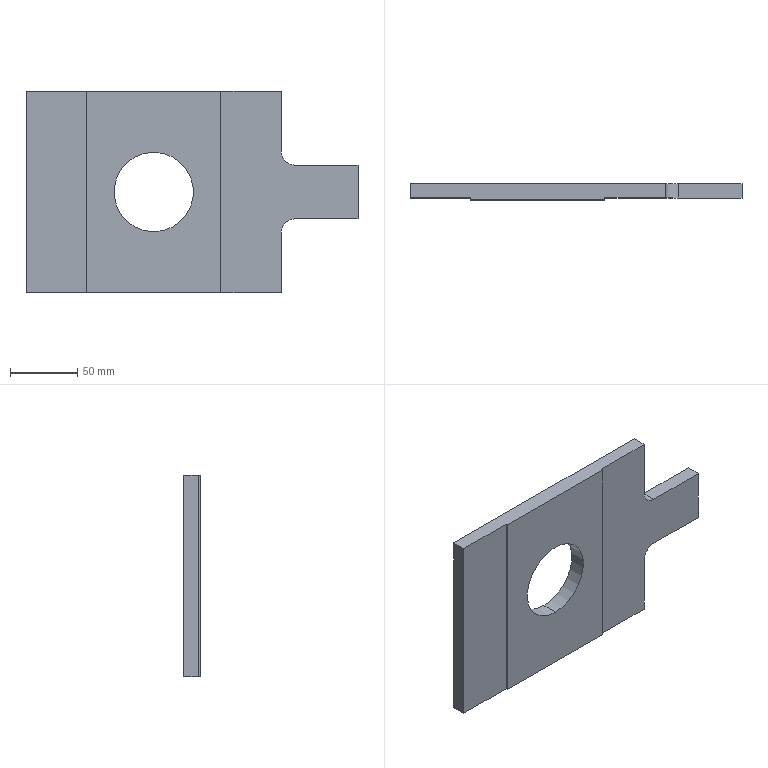Part | SolidWorks | features ICE 2, Extrusion 1, Fillet 1 | 1 solid | 18 faces | box 247 x 12 x 150 mm | volume 313333 mm3 | plane 14 | cylinder 4 | commonest cylinder face diameters 20 x2 59 x2
STEP:
#1=CARTESIAN_POINT('',(0.,0.,29.5));
#2=VERTEX_POINT('',#1);
#3=CARTESIAN_POINT('',(0.,0.,-29.5));
#4=VERTEX_POINT('',#3);
#5=CARTESIAN_POINT('',(0.,0.,0.));
#6=DIRECTION('',(0.,-1.,0.));
#7=DIRECTION('',(0.,0.,1.));
#8=AXIS2_PLACEMENT_3D('',#5,#6,#7);
#9=CIRCLE('',#8,29.5);
#10=EDGE_CURVE('',#2,#4,#9,.T.);
#11=ORIENTED_EDGE('',*,*,#10,.T.);
#12=CARTESIAN_POINT('',(0.,12.,-29.5));
#13=VERTEX_POINT('',#12);
#14=CARTESIAN_POINT('',(0.,-0.001,-29.5));
#15=DIRECTION('',(0.,1.,0.));
#16=VECTOR('',#15,1000.);
#17=LINE('',#14,#16);
#18=EDGE_CURVE('',#4,#13,#17,.T.);
#19=ORIENTED_EDGE('',*,*,#18,.T.);
#20=CARTESIAN_POINT('',(0.,12.,29.5));
#21=VERTEX_POINT('',#20);
#22=CARTESIAN_POINT('',(0.,12.,0.));
#23=DIRECTION('',(0.,1.,0.));
#24=DIRECTION('',(0.,0.,1.));
#25=AXIS2_PLACEMENT_3D('',#22,#23,#24);
#26=CIRCLE('',#25,29.5);
#27=EDGE_CURVE('',#13,#21,#26,.T.);
#28=ORIENTED_EDGE('',*,*,#27,.T.);
#29=CARTESIAN_POINT('',(0.,-0.001,29.5));
#30=DIRECTION('',(0.,1.,0.));
#31=VECTOR('',#30,1000.);
#32=LINE('',#29,#31);
#33=EDGE_CURVE('',#2,#21,#32,.T.);
#34=ORIENTED_EDGE('',*,*,#33,.F.);
#35=EDGE_LOOP('',(#11,#19,#28,#34));
#36=FACE_OUTER_BOUND('',#35,.T.);
#37=CARTESIAN_POINT('',(0.,-0.001,0.));
#38=DIRECTION('',(0.,1.,0.));
#39=DIRECTION('',(0.,0.,1.));
#40=AXIS2_PLACEMENT_3D('',#37,#38,#39);
#41=CYLINDRICAL_SURFACE('',#40,29.5);
#42=ADVANCED_FACE('',(#36),#41,.F.);
#43=CARTESIAN_POINT('',(95.,1.5,75.));
#44=VERTEX_POINT('',#43);
#45=CARTESIAN_POINT('',(95.,1.5,30.));
#46=VERTEX_POINT('',#45);
#47=CARTESIAN_POINT('',(95.,1.5,75.));
#48=DIRECTION('',(0.,0.,-1.));
#49=VECTOR('',#48,1000.);
#50=LINE('',#47,#49);
#51=EDGE_CURVE('',#44,#46,#50,.T.);
#52=ORIENTED_EDGE('',*,*,#51,.T.);
#53=CARTESIAN_POINT('',(95.,12.,30.));
#54=VERTEX_POINT('',#53);
#55=CARTESIAN_POINT('',(95.,12.,30.));
#56=DIRECTION('',(0.,1.,0.));
#57=VECTOR('',#56,1000.);
#58=LINE('',#55,#57);
#59=EDGE_CURVE('',#46,#54,#58,.T.);
#60=ORIENTED_EDGE('',*,*,#59,.T.);
#61=CARTESIAN_POINT('',(95.,12.,75.));
#62=VERTEX_POINT('',#61);
#63=CARTESIAN_POINT('',(95.,12.,75.));
#64=DIRECTION('',(0.,0.,-1.));
#65=VECTOR('',#64,1000.);
#66=LINE('',#63,#65);
#67=EDGE_CURVE('',#62,#54,#66,.T.);
#68=ORIENTED_EDGE('',*,*,#67,.F.);
#69=CARTESIAN_POINT('',(95.,12.,75.));
#70=DIRECTION('',(0.,1.,0.));
#71=VECTOR('',#70,1000.);
#72=LINE('',#69,#71);
#73=EDGE_CURVE('',#44,#62,#72,.T.);
#74=ORIENTED_EDGE('',*,*,#73,.F.);
#75=EDGE_LOOP('',(#52,#60,#68,#74));
#76=FACE_OUTER_BOUND('',#75,.T.);
#77=CARTESIAN_POINT('',(95.,12.,75.));
#78=DIRECTION('',(-1.,0.,0.));
#79=DIRECTION('',(0.,0.,1.));
#80=AXIS2_PLACEMENT_3D('',#77,#78,#79);
#81=PLANE('',#80);
#82=ADVANCED_FACE('',(#76),#81,.F.);
#83=CARTESIAN_POINT('',(95.,12.,-30.));
#84=VERTEX_POINT('',#83);
#85=CARTESIAN_POINT('',(95.,12.,-75.));
#86=VERTEX_POINT('',#85);
#87=CARTESIAN_POINT('',(95.,12.,75.));
#88=DIRECTION('',(0.,0.,-1.));
#89=VECTOR('',#88,1000.);
#90=LINE('',#87,#89);
#91=EDGE_CURVE('',#84,#86,#90,.T.);
#92=ORIENTED_EDGE('',*,*,#91,.F.);
#93=CARTESIAN_POINT('',(95.,1.5,-30.));
#94=VERTEX_POINT('',#93);
#95=CARTESIAN_POINT('',(95.,1.5,-30.));
#96=DIRECTION('',(0.,-1.,0.));
#97=VECTOR('',#96,1000.);
#98=LINE('',#95,#97);
#99=EDGE_CURVE('',#84,#94,#98,.T.);
#100=ORIENTED_EDGE('',*,*,#99,.T.);
#101=CARTESIAN_POINT('',(95.,1.5,-75.));
#102=VERTEX_POINT('',#101);
#103=CARTESIAN_POINT('',(95.,1.5,75.));
#104=DIRECTION('',(0.,0.,-1.));
#105=VECTOR('',#104,1000.);
#106=LINE('',#103,#105);
#107=EDGE_CURVE('',#94,#102,#106,.T.);
#108=ORIENTED_EDGE('',*,*,#107,.T.);
#109=CARTESIAN_POINT('',(95.,12.,-75.));
#110=DIRECTION('',(0.,1.,0.));
#111=VECTOR('',#110,1000.);
#112=LINE('',#109,#111);
#113=EDGE_CURVE('',#102,#86,#112,.T.);
#114=ORIENTED_EDGE('',*,*,#113,.T.);
#115=EDGE_LOOP('',(#92,#100,#108,#114));
#116=FACE_OUTER_BOUND('',#115,.T.);
#117=CARTESIAN_POINT('',(95.,12.,75.));
#118=DIRECTION('',(-1.,0.,0.));
#119=DIRECTION('',(0.,0.,1.));
#120=AXIS2_PLACEMENT_3D('',#117,#118,#119);
#121=PLANE('',#120);
#122=ADVANCED_FACE('',(#116),#121,.F.);
#123=CARTESIAN_POINT('',(50.,0.,-75.));
#124=VERTEX_POINT('',#123);
#125=CARTESIAN_POINT('',(50.,1.5,-75.));
#126=VERTEX_POINT('',#125);
#127=CARTESIAN_POINT('',(50.,1.5,-75.));
#128=DIRECTION('',(0.,1.,0.));
#129=VECTOR('',#128,1000.);
#130=LINE('',#127,#129);
#131=EDGE_CURVE('',#124,#126,#130,.T.);
#132=ORIENTED_EDGE('',*,*,#131,.T.);
#133=CARTESIAN_POINT('',(50.,1.5,75.));
#134=VERTEX_POINT('',#133);
#135=CARTESIAN_POINT('',(50.,1.5,75.));
#136=DIRECTION('',(0.,0.,-1.));
#137=VECTOR('',#136,1000.);
#138=LINE('',#135,#137);
#139=EDGE_CURVE('',#134,#126,#138,.T.);
#140=ORIENTED_EDGE('',*,*,#139,.F.);
#141=CARTESIAN_POINT('',(50.,0.,75.));
#142=VERTEX_POINT('',#141);
#143=CARTESIAN_POINT('',(50.,1.5,75.));
#144=DIRECTION('',(0.,1.,0.));
#145=VECTOR('',#144,1000.);
#146=LINE('',#143,#145);
#147=EDGE_CURVE('',#142,#134,#146,.T.);
#148=ORIENTED_EDGE('',*,*,#147,.F.);
#149=CARTESIAN_POINT('',(50.,0.,75.));
#150=DIRECTION('',(0.,0.,-1.));
#151=VECTOR('',#150,1000.);
#152=LINE('',#149,#151);
#153=EDGE_CURVE('',#142,#124,#152,.T.);
#154=ORIENTED_EDGE('',*,*,#153,.T.);
#155=EDGE_LOOP('',(#132,#140,#148,#154));
#156=FACE_OUTER_BOUND('',#155,.T.);
#157=CARTESIAN_POINT('',(50.,1.5,75.));
#158=DIRECTION('',(-1.,0.,0.));
#159=DIRECTION('',(0.,0.,1.));
#160=AXIS2_PLACEMENT_3D('',#157,#158,#159);
#161=PLANE('',#160);
#162=ADVANCED_FACE('',(#156),#161,.F.);
#163=CARTESIAN_POINT('',(95.,1.5,-75.));
#164=DIRECTION('',(1.,0.,0.));
#165=VECTOR('',#164,1000.);
#166=LINE('',#163,#165);
#167=EDGE_CURVE('',#126,#102,#166,.T.);
#168=ORIENTED_EDGE('',*,*,#167,.T.);
#169=ORIENTED_EDGE('',*,*,#107,.F.);
#170=CARTESIAN_POINT('',(105.,1.5,-20.));
#171=VERTEX_POINT('',#170);
#172=CARTESIAN_POINT('',(105.,1.5,-30.));
#173=DIRECTION('',(0.,1.,0.));
#174=DIRECTION('',(0.,0.,1.));
#175=AXIS2_PLACEMENT_3D('',#172,#173,#174);
#176=CIRCLE('',#175,10.);
#177=EDGE_CURVE('',#94,#171,#176,.T.);
#178=ORIENTED_EDGE('',*,*,#177,.T.);
#179=CARTESIAN_POINT('',(152.,1.5,-20.));
#180=VERTEX_POINT('',#179);
#181=CARTESIAN_POINT('',(152.,1.5,-20.));
#182=DIRECTION('',(-1.,0.,0.));
#183=VECTOR('',#182,1000.);
#184=LINE('',#181,#183);
#185=EDGE_CURVE('',#180,#171,#184,.T.);
#186=ORIENTED_EDGE('',*,*,#185,.F.);
#187=CARTESIAN_POINT('',(152.,1.5,20.));
#188=VERTEX_POINT('',#187);
#189=CARTESIAN_POINT('',(152.,1.5,20.));
#190=DIRECTION('',(0.,0.,-1.));
#191=VECTOR('',#190,1000.);
#192=LINE('',#189,#191);
#193=EDGE_CURVE('',#188,#180,#192,.T.);
#194=ORIENTED_EDGE('',*,*,#193,.F.);
#195=CARTESIAN_POINT('',(105.,1.5,20.));
#196=VERTEX_POINT('',#195);
#197=CARTESIAN_POINT('',(152.,1.5,20.));
#198=DIRECTION('',(-1.,0.,0.));
#199=VECTOR('',#198,1000.);
#200=LINE('',#197,#199);
#201=EDGE_CURVE('',#188,#196,#200,.T.);
#202=ORIENTED_EDGE('',*,*,#201,.T.);
#203=CARTESIAN_POINT('',(105.,1.5,30.));
#204=DIRECTION('',(0.,1.,0.));
#205=DIRECTION('',(0.,0.,1.));
#206=AXIS2_PLACEMENT_3D('',#203,#204,#205);
#207=CIRCLE('',#206,10.);
#208=EDGE_CURVE('',#196,#46,#207,.T.);
#209=ORIENTED_EDGE('',*,*,#208,.T.);
#210=ORIENTED_EDGE('',*,*,#51,.F.);
#211=CARTESIAN_POINT('',(95.,1.5,75.));
#212=DIRECTION('',(1.,0.,0.));
#213=VECTOR('',#212,1000.);
#214=LINE('',#211,#213);
#215=EDGE_CURVE('',#134,#44,#214,.T.);
#216=ORIENTED_EDGE('',*,*,#215,.F.);
#217=ORIENTED_EDGE('',*,*,#139,.T.);
#218=EDGE_LOOP('',(#168,#169,#178,#186,#194,#202,#209,#210,#216,#217));
#219=FACE_OUTER_BOUND('',#218,.T.);
#220=CARTESIAN_POINT('',(95.,1.5,75.));
#221=DIRECTION('',(0.,1.,0.));
#222=DIRECTION('',(0.,0.,1.));
#223=AXIS2_PLACEMENT_3D('',#220,#221,#222);
#224=PLANE('',#223);
#225=ADVANCED_FACE('',(#219),#224,.F.);
#226=CARTESIAN_POINT('',(0.,12.,0.));
#227=DIRECTION('',(0.,1.,0.));
#228=DIRECTION('',(0.,0.,1.));
#229=AXIS2_PLACEMENT_3D('',#226,#227,#228);
#230=CIRCLE('',#229,29.5);
#231=EDGE_CURVE('',#21,#13,#230,.T.);
#232=ORIENTED_EDGE('',*,*,#231,.F.);
#233=ORIENTED_EDGE('',*,*,#27,.F.);
#234=EDGE_LOOP('',(#232,#233));
#235=FACE_BOUND('',#234,.T.);
#236=CARTESIAN_POINT('',(-95.,12.,-75.));
#237=VERTEX_POINT('',#236);
#238=CARTESIAN_POINT('',(-95.,12.,-75.));
#239=DIRECTION('',(-1.,0.,0.));
#240=VECTOR('',#239,1000.);
#241=LINE('',#238,#240);
#242=EDGE_CURVE('',#86,#237,#241,.T.);
#243=ORIENTED_EDGE('',*,*,#242,.T.);
#244=CARTESIAN_POINT('',(-95.,12.,75.));
#245=VERTEX_POINT('',#244);
#246=CARTESIAN_POINT('',(-95.,12.,75.));
#247=DIRECTION('',(0.,0.,-1.));
#248=VECTOR('',#247,1000.);
#249=LINE('',#246,#248);
#250=EDGE_CURVE('',#245,#237,#249,.T.);
#251=ORIENTED_EDGE('',*,*,#250,.F.);
#252=CARTESIAN_POINT('',(-95.,12.,75.));
#253=DIRECTION('',(-1.,0.,0.));
#254=VECTOR('',#253,1000.);
#255=LINE('',#252,#254);
#256=EDGE_CURVE('',#62,#245,#255,.T.);
#257=ORIENTED_EDGE('',*,*,#256,.F.);
#258=ORIENTED_EDGE('',*,*,#67,.T.);
#259=CARTESIAN_POINT('',(105.,12.,20.));
#260=VERTEX_POINT('',#259);
#261=CARTESIAN_POINT('',(105.,12.,30.));
#262=DIRECTION('',(0.,-1.,0.));
#263=DIRECTION('',(0.,0.,-1.));
#264=AXIS2_PLACEMENT_3D('',#261,#262,#263);
#265=CIRCLE('',#264,10.);
#266=EDGE_CURVE('',#54,#260,#265,.T.);
#267=ORIENTED_EDGE('',*,*,#266,.T.);
#268=CARTESIAN_POINT('',(152.,12.,20.));
#269=VERTEX_POINT('',#268);
#270=CARTESIAN_POINT('',(152.,12.,20.));
#271=DIRECTION('',(-1.,0.,0.));
#272=VECTOR('',#271,1000.);
#273=LINE('',#270,#272);
#274=EDGE_CURVE('',#269,#260,#273,.T.);
#275=ORIENTED_EDGE('',*,*,#274,.F.);
#276=CARTESIAN_POINT('',(152.,12.,-20.));
#277=VERTEX_POINT('',#276);
#278=CARTESIAN_POINT('',(152.,12.,20.));
#279=DIRECTION('',(0.,0.,1.));
#280=VECTOR('',#279,1000.);
#281=LINE('',#278,#280);
#282=EDGE_CURVE('',#277,#269,#281,.T.);
#283=ORIENTED_EDGE('',*,*,#282,.F.);
#284=CARTESIAN_POINT('',(105.,12.,-20.));
#285=VERTEX_POINT('',#284);
#286=CARTESIAN_POINT('',(152.,12.,-20.));
#287=DIRECTION('',(-1.,0.,0.));
#288=VECTOR('',#287,1000.);
#289=LINE('',#286,#288);
#290=EDGE_CURVE('',#277,#285,#289,.T.);
#291=ORIENTED_EDGE('',*,*,#290,.T.);
#292=CARTESIAN_POINT('',(105.,12.,-30.));
#293=DIRECTION('',(0.,-1.,0.));
#294=DIRECTION('',(0.,0.,-1.));
#295=AXIS2_PLACEMENT_3D('',#292,#293,#294);
#296=CIRCLE('',#295,10.);
#297=EDGE_CURVE('',#285,#84,#296,.T.);
#298=ORIENTED_EDGE('',*,*,#297,.T.);
#299=ORIENTED_EDGE('',*,*,#91,.T.);
#300=EDGE_LOOP('',(#243,#251,#257,#258,#267,#275,#283,#291,#298,#299));
#301=FACE_OUTER_BOUND('',#300,.T.);
#302=CARTESIAN_POINT('',(-95.,12.,75.));
#303=DIRECTION('',(0.,-1.,0.));
#304=DIRECTION('',(0.,0.,-1.));
#305=AXIS2_PLACEMENT_3D('',#302,#303,#304);
#306=PLANE('',#305);
#307=ADVANCED_FACE('',(#235,#301),#306,.F.);
#308=CARTESIAN_POINT('',(-95.,1.5,-75.));
#309=VERTEX_POINT('',#308);
#310=CARTESIAN_POINT('',(-95.,1.5,-75.));
#311=DIRECTION('',(0.,-1.,0.));
#312=VECTOR('',#311,1000.);
#313=LINE('',#310,#312);
#314=EDGE_CURVE('',#237,#309,#313,.T.);
#315=ORIENTED_EDGE('',*,*,#314,.T.);
#316=CARTESIAN_POINT('',(-95.,1.5,75.));
#317=VERTEX_POINT('',#316);
#318=CARTESIAN_POINT('',(-95.,1.5,75.));
#319=DIRECTION('',(0.,0.,-1.));
#320=VECTOR('',#319,1000.);
#321=LINE('',#318,#320);
#322=EDGE_CURVE('',#317,#309,#321,.T.);
#323=ORIENTED_EDGE('',*,*,#322,.F.);
#324=CARTESIAN_POINT('',(-95.,1.5,75.));
#325=DIRECTION('',(0.,-1.,0.));
#326=VECTOR('',#325,1000.);
#327=LINE('',#324,#326);
#328=EDGE_CURVE('',#245,#317,#327,.T.);
#329=ORIENTED_EDGE('',*,*,#328,.F.);
#330=ORIENTED_EDGE('',*,*,#250,.T.);
#331=EDGE_LOOP('',(#315,#323,#329,#330));
#332=FACE_OUTER_BOUND('',#331,.T.);
#333=CARTESIAN_POINT('',(-95.,1.5,75.));
#334=DIRECTION('',(1.,0.,0.));
#335=DIRECTION('',(0.,0.,-1.));
#336=AXIS2_PLACEMENT_3D('',#333,#334,#335);
#337=PLANE('',#336);
#338=ADVANCED_FACE('',(#332),#337,.F.);
#339=CARTESIAN_POINT('',(-50.,1.5,-75.));
#340=VERTEX_POINT('',#339);
#341=CARTESIAN_POINT('',(-50.,1.5,-75.));
#342=DIRECTION('',(1.,0.,0.));
#343=VECTOR('',#342,1000.);
#344=LINE('',#341,#343);
#345=EDGE_CURVE('',#309,#340,#344,.T.);
#346=ORIENTED_EDGE('',*,*,#345,.T.);
#347=CARTESIAN_POINT('',(-50.,1.5,75.));
#348=VERTEX_POINT('',#347);
#349=CARTESIAN_POINT('',(-50.,1.5,75.));
#350=DIRECTION('',(0.,0.,-1.));
#351=VECTOR('',#350,1000.);
#352=LINE('',#349,#351);
#353=EDGE_CURVE('',#348,#340,#352,.T.);
#354=ORIENTED_EDGE('',*,*,#353,.F.);
#355=CARTESIAN_POINT('',(-50.,1.5,75.));
#356=DIRECTION('',(1.,0.,0.));
#357=VECTOR('',#356,1000.);
#358=LINE('',#355,#357);
#359=EDGE_CURVE('',#317,#348,#358,.T.);
#360=ORIENTED_EDGE('',*,*,#359,.F.);
#361=ORIENTED_EDGE('',*,*,#322,.T.);
#362=EDGE_LOOP('',(#346,#354,#360,#361));
#363=FACE_OUTER_BOUND('',#362,.T.);
#364=CARTESIAN_POINT('',(-50.,1.5,75.));
#365=DIRECTION('',(0.,1.,0.));
#366=DIRECTION('',(0.,0.,1.));
#367=AXIS2_PLACEMENT_3D('',#364,#365,#366);
#368=PLANE('',#367);
#369=ADVANCED_FACE('',(#363),#368,.F.);
#370=CARTESIAN_POINT('',(-50.,0.,-75.));
#371=VERTEX_POINT('',#370);
#372=CARTESIAN_POINT('',(-50.,0.,-75.));
#373=DIRECTION('',(0.,-1.,0.));
#374=VECTOR('',#373,1000.);
#375=LINE('',#372,#374);
#376=EDGE_CURVE('',#340,#371,#375,.T.);
#377=ORIENTED_EDGE('',*,*,#376,.T.);
#378=CARTESIAN_POINT('',(-50.,0.,75.));
#379=VERTEX_POINT('',#378);
#380=CARTESIAN_POINT('',(-50.,0.,75.));
#381=DIRECTION('',(0.,0.,-1.));
#382=VECTOR('',#381,1000.);
#383=LINE('',#380,#382);
#384=EDGE_CURVE('',#379,#371,#383,.T.);
#385=ORIENTED_EDGE('',*,*,#384,.F.);
#386=CARTESIAN_POINT('',(-50.,0.,75.));
#387=DIRECTION('',(0.,-1.,0.));
#388=VECTOR('',#387,1000.);
#389=LINE('',#386,#388);
#390=EDGE_CURVE('',#348,#379,#389,.T.);
#391=ORIENTED_EDGE('',*,*,#390,.F.);
#392=ORIENTED_EDGE('',*,*,#353,.T.);
#393=EDGE_LOOP('',(#377,#385,#391,#392));
#394=FACE_OUTER_BOUND('',#393,.T.);
#395=CARTESIAN_POINT('',(-50.,0.,75.));
#396=DIRECTION('',(1.,0.,0.));
#397=DIRECTION('',(0.,1.,0.));
#398=AXIS2_PLACEMENT_3D('',#395,#396,#397);
#399=PLANE('',#398);
#400=ADVANCED_FACE('',(#394),#399,.F.);
#401=ORIENTED_EDGE('',*,*,#10,.F.);
#402=CARTESIAN_POINT('',(0.,0.,0.));
#403=DIRECTION('',(0.,-1.,0.));
#404=DIRECTION('',(0.,0.,1.));
#405=AXIS2_PLACEMENT_3D('',#402,#403,#404);
#406=CIRCLE('',#405,29.5);
#407=EDGE_CURVE('',#4,#2,#406,.T.);
#408=ORIENTED_EDGE('',*,*,#407,.F.);
#409=EDGE_LOOP('',(#401,#408));
#410=FACE_BOUND('',#409,.T.);
#411=CARTESIAN_POINT('',(0.,0.,-75.));
#412=DIRECTION('',(1.,0.,0.));
#413=VECTOR('',#412,1000.);
#414=LINE('',#411,#413);
#415=EDGE_CURVE('',#371,#124,#414,.T.);
#416=ORIENTED_EDGE('',*,*,#415,.T.);
#417=ORIENTED_EDGE('',*,*,#153,.F.);
#418=CARTESIAN_POINT('',(50.,0.,75.));
#419=DIRECTION('',(1.,0.,0.));
#420=VECTOR('',#419,1000.);
#421=LINE('',#418,#420);
#422=EDGE_CURVE('',#379,#142,#421,.T.);
#423=ORIENTED_EDGE('',*,*,#422,.F.);
#424=ORIENTED_EDGE('',*,*,#384,.T.);
#425=EDGE_LOOP('',(#416,#417,#423,#424));
#426=FACE_OUTER_BOUND('',#425,.T.);
#427=CARTESIAN_POINT('',(0.,0.,75.));
#428=DIRECTION('',(0.,1.,0.));
#429=DIRECTION('',(0.,0.,1.));
#430=AXIS2_PLACEMENT_3D('',#427,#428,#429);
#431=PLANE('',#430);
#432=ADVANCED_FACE('',(#410,#426),#431,.F.);
#433=ORIENTED_EDGE('',*,*,#422,.T.);
#434=ORIENTED_EDGE('',*,*,#147,.T.);
#435=ORIENTED_EDGE('',*,*,#215,.T.);
#436=ORIENTED_EDGE('',*,*,#73,.T.);
#437=ORIENTED_EDGE('',*,*,#256,.T.);
#438=ORIENTED_EDGE('',*,*,#328,.T.);
#439=ORIENTED_EDGE('',*,*,#359,.T.);
#440=ORIENTED_EDGE('',*,*,#390,.T.);
#441=EDGE_LOOP('',(#433,#434,#435,#436,#437,#438,#439,#440));
#442=FACE_OUTER_BOUND('',#441,.T.);
#443=CARTESIAN_POINT('',(0.,0.,75.));
#444=DIRECTION('',(0.,0.,-1.));
#445=DIRECTION('',(-1.,0.,0.));
#446=AXIS2_PLACEMENT_3D('',#443,#444,#445);
#447=PLANE('',#446);
#448=ADVANCED_FACE('',(#442),#447,.F.);
#449=ORIENTED_EDGE('',*,*,#131,.F.);
#450=ORIENTED_EDGE('',*,*,#415,.F.);
#451=ORIENTED_EDGE('',*,*,#376,.F.);
#452=ORIENTED_EDGE('',*,*,#345,.F.);
#453=ORIENTED_EDGE('',*,*,#314,.F.);
#454=ORIENTED_EDGE('',*,*,#242,.F.);
#455=ORIENTED_EDGE('',*,*,#113,.F.);
#456=ORIENTED_EDGE('',*,*,#167,.F.);
#457=EDGE_LOOP('',(#449,#450,#451,#452,#453,#454,#455,#456));
#458=FACE_OUTER_BOUND('',#457,.T.);
#459=CARTESIAN_POINT('',(0.,0.,-75.));
#460=DIRECTION('',(0.,0.,-1.));
#461=DIRECTION('',(-1.,0.,0.));
#462=AXIS2_PLACEMENT_3D('',#459,#460,#461);
#463=PLANE('',#462);
#464=ADVANCED_FACE('',(#458),#463,.T.);
#465=ORIENTED_EDGE('',*,*,#18,.F.);
#466=ORIENTED_EDGE('',*,*,#407,.T.);
#467=ORIENTED_EDGE('',*,*,#33,.T.);
#468=ORIENTED_EDGE('',*,*,#231,.T.);
#469=EDGE_LOOP('',(#465,#466,#467,#468));
#470=FACE_OUTER_BOUND('',#469,.T.);
#471=CARTESIAN_POINT('',(0.,-0.001,0.));
#472=DIRECTION('',(0.,1.,0.));
#473=DIRECTION('',(0.,0.,1.));
#474=AXIS2_PLACEMENT_3D('',#471,#472,#473);
#475=CYLINDRICAL_SURFACE('',#474,29.5);
#476=ADVANCED_FACE('',(#470),#475,.F.);
#477=ORIENTED_EDGE('',*,*,#274,.T.);
#478=CARTESIAN_POINT('',(105.,1.5,20.));
#479=DIRECTION('',(0.,-1.,0.));
#480=VECTOR('',#479,1000.);
#481=LINE('',#478,#480);
#482=EDGE_CURVE('',#260,#196,#481,.T.);
#483=ORIENTED_EDGE('',*,*,#482,.T.);
#484=ORIENTED_EDGE('',*,*,#201,.F.);
#485=CARTESIAN_POINT('',(152.,12.,20.));
#486=DIRECTION('',(0.,-1.,0.));
#487=VECTOR('',#486,1000.);
#488=LINE('',#485,#487);
#489=EDGE_CURVE('',#269,#188,#488,.T.);
#490=ORIENTED_EDGE('',*,*,#489,.F.);
#491=EDGE_LOOP('',(#477,#483,#484,#490));
#492=FACE_OUTER_BOUND('',#491,.T.);
#493=CARTESIAN_POINT('',(152.,12.,20.));
#494=DIRECTION('',(0.,0.,-1.));
#495=DIRECTION('',(-1.,0.,0.));
#496=AXIS2_PLACEMENT_3D('',#493,#494,#495);
#497=PLANE('',#496);
#498=ADVANCED_FACE('',(#492),#497,.F.);
#499=ORIENTED_EDGE('',*,*,#185,.T.);
#500=CARTESIAN_POINT('',(105.,12.,-20.));
#501=DIRECTION('',(0.,1.,0.));
#502=VECTOR('',#501,1000.);
#503=LINE('',#500,#502);
#504=EDGE_CURVE('',#171,#285,#503,.T.);
#505=ORIENTED_EDGE('',*,*,#504,.T.);
#506=ORIENTED_EDGE('',*,*,#290,.F.);
#507=CARTESIAN_POINT('',(152.,12.,-20.));
#508=DIRECTION('',(0.,1.,0.));
#509=VECTOR('',#508,1000.);
#510=LINE('',#507,#509);
#511=EDGE_CURVE('',#180,#277,#510,.T.);
#512=ORIENTED_EDGE('',*,*,#511,.F.);
#513=EDGE_LOOP('',(#499,#505,#506,#512));
#514=FACE_OUTER_BOUND('',#513,.T.);
#515=CARTESIAN_POINT('',(152.,12.,-20.));
#516=DIRECTION('',(0.,0.,1.));
#517=DIRECTION('',(1.,0.,0.));
#518=AXIS2_PLACEMENT_3D('',#515,#516,#517);
#519=PLANE('',#518);
#520=ADVANCED_FACE('',(#514),#519,.F.);
#521=ORIENTED_EDGE('',*,*,#489,.T.);
#522=ORIENTED_EDGE('',*,*,#193,.T.);
#523=ORIENTED_EDGE('',*,*,#511,.T.);
#524=ORIENTED_EDGE('',*,*,#282,.T.);
#525=EDGE_LOOP('',(#521,#522,#523,#524));
#526=FACE_OUTER_BOUND('',#525,.T.);
#527=CARTESIAN_POINT('',(152.,0.,0.));
#528=DIRECTION('',(1.,0.,0.));
#529=DIRECTION('',(0.,0.,-1.));
#530=AXIS2_PLACEMENT_3D('',#527,#528,#529);
#531=PLANE('',#530);
#532=ADVANCED_FACE('',(#526),#531,.T.);
#533=ORIENTED_EDGE('',*,*,#177,.F.);
#534=ORIENTED_EDGE('',*,*,#99,.F.);
#535=ORIENTED_EDGE('',*,*,#297,.F.);
#536=ORIENTED_EDGE('',*,*,#504,.F.);
#537=EDGE_LOOP('',(#533,#534,#535,#536));
#538=FACE_OUTER_BOUND('',#537,.T.);
#539=CARTESIAN_POINT('',(105.,12.,-30.));
#540=DIRECTION('',(0.,-1.,0.));
#541=DIRECTION('',(0.,0.,-1.));
#542=AXIS2_PLACEMENT_3D('',#539,#540,#541);
#543=CYLINDRICAL_SURFACE('',#542,10.);
#544=ADVANCED_FACE('',(#538),#543,.F.);
#545=ORIENTED_EDGE('',*,*,#266,.F.);
#546=ORIENTED_EDGE('',*,*,#59,.F.);
#547=ORIENTED_EDGE('',*,*,#208,.F.);
#548=ORIENTED_EDGE('',*,*,#482,.F.);
#549=EDGE_LOOP('',(#545,#546,#547,#548));
#550=FACE_OUTER_BOUND('',#549,.T.);
#551=CARTESIAN_POINT('',(105.,12.,30.));
#552=DIRECTION('',(0.,1.,0.));
#553=DIRECTION('',(0.,0.,1.));
#554=AXIS2_PLACEMENT_3D('',#551,#552,#553);
#555=CYLINDRICAL_SURFACE('',#554,10.);
#556=ADVANCED_FACE('',(#550),#555,.F.);
#557=CLOSED_SHELL('',(#42,#82,#122,#162,#225,#307,#338,#369,#400,#432,#448,#464,#476,#498,#520,#532,#544,#556));
#558=MANIFOLD_SOLID_BREP('',#557);
#559=CARTESIAN_POINT('',(0.,0.,0.));
#560=DIRECTION('',(0.,0.,1.));
#561=DIRECTION('',(1.,0.,0.));
#562=AXIS2_PLACEMENT_3D('',#559,#560,#561);
#563=(LENGTH_UNIT()NAMED_UNIT(*)SI_UNIT(.MILLI.,.METRE.));
#564=UNCERTAINTY_MEASURE_WITH_UNIT(LENGTH_MEASURE(0.00001),#563,'','');
#565=(NAMED_UNIT(*)PLANE_ANGLE_UNIT()SI_UNIT($,.RADIAN.));
#566=(NAMED_UNIT(*)SI_UNIT($,.STERADIAN.)SOLID_ANGLE_UNIT());
#567=(GEOMETRIC_REPRESENTATION_CONTEXT(3)GLOBAL_UNCERTAINTY_ASSIGNED_CONTEXT((#564))GLOBAL_UNIT_ASSIGNED_CONTEXT((#563,#565,#566))REPRESENTATION_CONTEXT('',''));
#568=ADVANCED_BREP_SHAPE_REPRESENTATION('',(#558,#562),#567);